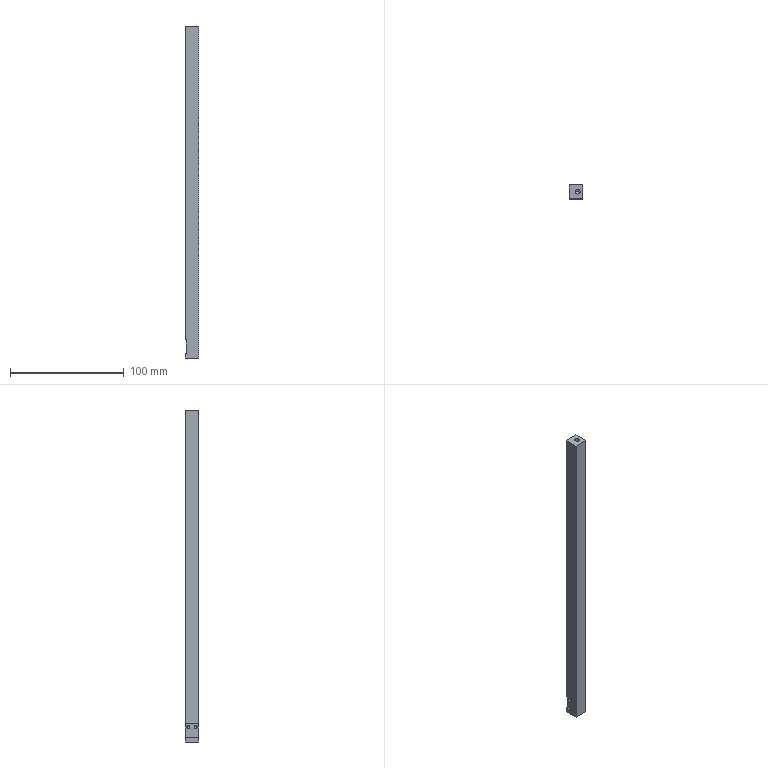Part | NX | features BREP 1 | 1 solid | 26 faces | box 12 x 12 x 292 mm | volume 41474 mm3 | plane 10 | cone 8 | cylinder 8 | commonest cylinder face diameters 2.5 x4 4.2 x4
STEP:
#1=CARTESIAN_POINT('',(-771.889,-6.832,13.662));
#2=VERTEX_POINT('',#1);
#3=CARTESIAN_POINT('',(-773.989,-6.832,12.4));
#4=VERTEX_POINT('',#3);
#5=CARTESIAN_POINT('',(-773.989,-6.832,12.4));
#6=DIRECTION('',(-0.8572,0.,-0.515));
#7=VECTOR('',#6,1000.);
#8=LINE('',#5,#7);
#9=EDGE_CURVE('',#2,#4,#8,.T.);
#10=ORIENTED_EDGE('',*,*,#9,.F.);
#11=CARTESIAN_POINT('',(-769.789,-6.832,12.4));
#12=VERTEX_POINT('',#11);
#13=CARTESIAN_POINT('',(-769.789,-6.832,12.4));
#14=DIRECTION('',(0.8572,0.,-0.515));
#15=VECTOR('',#14,1000.);
#16=LINE('',#13,#15);
#17=EDGE_CURVE('',#2,#12,#16,.T.);
#18=ORIENTED_EDGE('',*,*,#17,.T.);
#19=CARTESIAN_POINT('',(-770.231,-8.121,12.4));
#20=VERTEX_POINT('',#19);
#21=CARTESIAN_POINT('',(-771.889,-6.832,12.4));
#22=DIRECTION('',(0.,0.,-1.));
#23=DIRECTION('',(-1.,0.,0.));
#24=AXIS2_PLACEMENT_3D('',#21,#22,#23);
#25=CIRCLE('',#24,2.1);
#26=EDGE_CURVE('',#12,#20,#25,.T.);
#27=ORIENTED_EDGE('',*,*,#26,.T.);
#28=CARTESIAN_POINT('',(-773.546,-8.121,12.4));
#29=VERTEX_POINT('',#28);
#30=CARTESIAN_POINT('',(-773.546,-8.121,12.4));
#31=CARTESIAN_POINT('',(-773.126,-7.881,12.688));
#32=CARTESIAN_POINT('',(-771.895,-7.799,13.423));
#33=CARTESIAN_POINT('',(-770.654,-7.88,12.689));
#34=CARTESIAN_POINT('',(-770.231,-8.121,12.4));
#35=B_SPLINE_CURVE_WITH_KNOTS('',3,(#30,#31,#32,#33,#34),.UNSPECIFIED.,.F.,.F.,(4,1,4),(0.,0.5,1.),.UNSPECIFIED.);
#36=EDGE_CURVE('',#29,#20,#35,.T.);
#37=ORIENTED_EDGE('',*,*,#36,.F.);
#38=CARTESIAN_POINT('',(-771.889,-6.832,12.4));
#39=DIRECTION('',(0.,0.,-1.));
#40=DIRECTION('',(-1.,0.,0.));
#41=AXIS2_PLACEMENT_3D('',#38,#39,#40);
#42=CIRCLE('',#41,2.1);
#43=EDGE_CURVE('',#29,#4,#42,.T.);
#44=ORIENTED_EDGE('',*,*,#43,.T.);
#45=EDGE_LOOP('',(#10,#18,#27,#37,#44));
#46=FACE_BOUND('',#45,.T.);
#47=CARTESIAN_POINT('',(-771.889,-6.832,12.4));
#48=DIRECTION('',(0.,0.,-1.));
#49=DIRECTION('',(-1.,0.,0.));
#50=AXIS2_PLACEMENT_3D('',#47,#48,#49);
#51=CONICAL_SURFACE('',#50,2.1,1.03);
#52=ADVANCED_FACE('',(#46),#51,.F.);
#53=ORIENTED_EDGE('',*,*,#26,.F.);
#54=CARTESIAN_POINT('',(-769.789,-6.832,0.));
#55=VERTEX_POINT('',#54);
#56=CARTESIAN_POINT('',(-769.789,-6.832,0.));
#57=DIRECTION('',(0.,0.,-1.));
#58=VECTOR('',#57,1000.);
#59=LINE('',#56,#58);
#60=EDGE_CURVE('',#12,#55,#59,.T.);
#61=ORIENTED_EDGE('',*,*,#60,.T.);
#62=CARTESIAN_POINT('',(-773.989,-6.832,0.));
#63=VERTEX_POINT('',#62);
#64=CARTESIAN_POINT('',(-771.889,-6.832,0.));
#65=DIRECTION('',(0.,0.,-1.));
#66=DIRECTION('',(-1.,0.,0.));
#67=AXIS2_PLACEMENT_3D('',#64,#65,#66);
#68=CIRCLE('',#67,2.1);
#69=EDGE_CURVE('',#55,#63,#68,.T.);
#70=ORIENTED_EDGE('',*,*,#69,.T.);
#71=CARTESIAN_POINT('',(-773.989,-6.832,0.));
#72=DIRECTION('',(0.,0.,-1.));
#73=VECTOR('',#72,1000.);
#74=LINE('',#71,#73);
#75=EDGE_CURVE('',#4,#63,#74,.T.);
#76=ORIENTED_EDGE('',*,*,#75,.F.);
#77=ORIENTED_EDGE('',*,*,#43,.F.);
#78=CARTESIAN_POINT('',(-773.546,-8.121,12.4));
#79=CARTESIAN_POINT('',(-773.403,-8.305,12.179));
#80=CARTESIAN_POINT('',(-772.89,-8.778,11.952));
#81=CARTESIAN_POINT('',(-771.888,-9.009,11.963));
#82=CARTESIAN_POINT('',(-770.887,-8.777,11.952));
#83=CARTESIAN_POINT('',(-770.374,-8.305,12.179));
#84=CARTESIAN_POINT('',(-770.231,-8.121,12.4));
#85=B_SPLINE_CURVE_WITH_KNOTS('',3,(#78,#79,#80,#81,#82,#83,#84),.UNSPECIFIED.,.F.,.F.,(4,1,1,1,4),(0.,0.25,0.5,0.75,1.),.UNSPECIFIED.);
#86=EDGE_CURVE('',#20,#29,#85,.F.);
#87=ORIENTED_EDGE('',*,*,#86,.F.);
#88=EDGE_LOOP('',(#53,#61,#70,#76,#77,#87));
#89=FACE_BOUND('',#88,.T.);
#90=CARTESIAN_POINT('',(-771.889,-6.832,0.));
#91=DIRECTION('',(0.,0.,-1.));
#92=DIRECTION('',(-1.,0.,0.));
#93=AXIS2_PLACEMENT_3D('',#90,#91,#92);
#94=CYLINDRICAL_SURFACE('',#93,2.1);
#95=ADVANCED_FACE('',(#89),#94,.F.);
#96=CARTESIAN_POINT('',(-772.489,-5.832,279.6));
#97=VERTEX_POINT('',#96);
#98=CARTESIAN_POINT('',(-768.289,-5.832,279.6));
#99=VERTEX_POINT('',#98);
#100=CARTESIAN_POINT('',(-770.389,-5.832,279.6));
#101=DIRECTION('',(0.,0.,1.));
#102=DIRECTION('',(1.,0.,0.));
#103=AXIS2_PLACEMENT_3D('',#100,#101,#102);
#104=CIRCLE('',#103,2.1);
#105=EDGE_CURVE('',#97,#99,#104,.T.);
#106=ORIENTED_EDGE('',*,*,#105,.F.);
#107=CARTESIAN_POINT('',(-772.489,-5.832,292.));
#108=VERTEX_POINT('',#107);
#109=CARTESIAN_POINT('',(-772.489,-5.832,292.));
#110=DIRECTION('',(0.,0.,1.));
#111=VECTOR('',#110,1000.);
#112=LINE('',#109,#111);
#113=EDGE_CURVE('',#108,#97,#112,.F.);
#114=ORIENTED_EDGE('',*,*,#113,.F.);
#115=CARTESIAN_POINT('',(-768.289,-5.832,292.));
#116=VERTEX_POINT('',#115);
#117=CARTESIAN_POINT('',(-770.389,-5.832,292.));
#118=DIRECTION('',(0.,0.,1.));
#119=DIRECTION('',(1.,0.,0.));
#120=AXIS2_PLACEMENT_3D('',#117,#118,#119);
#121=CIRCLE('',#120,2.1);
#122=EDGE_CURVE('',#108,#116,#121,.T.);
#123=ORIENTED_EDGE('',*,*,#122,.T.);
#124=CARTESIAN_POINT('',(-768.289,-5.832,292.));
#125=DIRECTION('',(0.,0.,1.));
#126=VECTOR('',#125,1000.);
#127=LINE('',#124,#126);
#128=EDGE_CURVE('',#116,#99,#127,.F.);
#129=ORIENTED_EDGE('',*,*,#128,.T.);
#130=EDGE_LOOP('',(#106,#114,#123,#129));
#131=FACE_BOUND('',#130,.T.);
#132=CARTESIAN_POINT('',(-770.389,-5.832,292.));
#133=DIRECTION('',(0.,0.,1.));
#134=DIRECTION('',(1.,0.,0.));
#135=AXIS2_PLACEMENT_3D('',#132,#133,#134);
#136=CYLINDRICAL_SURFACE('',#135,2.1);
#137=ADVANCED_FACE('',(#131),#136,.F.);
#138=CARTESIAN_POINT('',(-770.389,-5.832,278.338));
#139=VERTEX_POINT('',#138);
#140=CARTESIAN_POINT('',(-768.289,-5.832,279.6));
#141=DIRECTION('',(0.8572,0.,0.515));
#142=VECTOR('',#141,1000.);
#143=LINE('',#140,#142);
#144=EDGE_CURVE('',#99,#139,#143,.F.);
#145=ORIENTED_EDGE('',*,*,#144,.T.);
#146=CARTESIAN_POINT('',(-772.489,-5.832,279.6));
#147=DIRECTION('',(-0.8572,0.,0.515));
#148=VECTOR('',#147,1000.);
#149=LINE('',#146,#148);
#150=EDGE_CURVE('',#97,#139,#149,.F.);
#151=ORIENTED_EDGE('',*,*,#150,.F.);
#152=ORIENTED_EDGE('',*,*,#105,.T.);
#153=EDGE_LOOP('',(#145,#151,#152));
#154=FACE_BOUND('',#153,.T.);
#155=CARTESIAN_POINT('',(-770.389,-5.832,279.6));
#156=DIRECTION('',(0.,0.,1.));
#157=DIRECTION('',(1.,0.,0.));
#158=AXIS2_PLACEMENT_3D('',#155,#156,#157);
#159=CONICAL_SURFACE('',#158,2.1,1.03);
#160=ADVANCED_FACE('',(#154),#159,.F.);
#161=CARTESIAN_POINT('',(-769.389,-9.082,11.95));
#162=VERTEX_POINT('',#161);
#163=CARTESIAN_POINT('',(-769.389,-9.082,14.45));
#164=VERTEX_POINT('',#163);
#165=CARTESIAN_POINT('',(-769.389,-9.082,13.2));
#166=DIRECTION('',(-1.,0.,0.));
#167=DIRECTION('',(0.,0.,1.));
#168=AXIS2_PLACEMENT_3D('',#165,#166,#167);
#169=CIRCLE('',#168,1.25);
#170=EDGE_CURVE('',#162,#164,#169,.T.);
#171=ORIENTED_EDGE('',*,*,#170,.F.);
#172=CARTESIAN_POINT('',(-776.889,-9.082,11.95));
#173=VERTEX_POINT('',#172);
#174=CARTESIAN_POINT('',(-776.889,-9.082,11.95));
#175=DIRECTION('',(-1.,0.,0.));
#176=VECTOR('',#175,1000.);
#177=LINE('',#174,#176);
#178=EDGE_CURVE('',#173,#162,#177,.F.);
#179=ORIENTED_EDGE('',*,*,#178,.F.);
#180=CARTESIAN_POINT('',(-776.889,-9.082,14.45));
#181=VERTEX_POINT('',#180);
#182=CARTESIAN_POINT('',(-776.889,-9.082,13.2));
#183=DIRECTION('',(-1.,0.,0.));
#184=DIRECTION('',(0.,0.,1.));
#185=AXIS2_PLACEMENT_3D('',#182,#183,#184);
#186=CIRCLE('',#185,1.25);
#187=EDGE_CURVE('',#173,#181,#186,.T.);
#188=ORIENTED_EDGE('',*,*,#187,.T.);
#189=CARTESIAN_POINT('',(-776.889,-9.082,14.45));
#190=DIRECTION('',(-1.,0.,0.));
#191=VECTOR('',#190,1000.);
#192=LINE('',#189,#191);
#193=EDGE_CURVE('',#181,#164,#192,.F.);
#194=ORIENTED_EDGE('',*,*,#193,.T.);
#195=EDGE_LOOP('',(#171,#179,#188,#194));
#196=FACE_BOUND('',#195,.T.);
#197=CARTESIAN_POINT('',(-776.889,-9.082,13.2));
#198=DIRECTION('',(-1.,0.,0.));
#199=DIRECTION('',(0.,0.,1.));
#200=AXIS2_PLACEMENT_3D('',#197,#198,#199);
#201=CYLINDRICAL_SURFACE('',#200,1.25);
#202=ADVANCED_FACE('',(#196),#201,.F.);
#203=CARTESIAN_POINT('',(-768.638,-9.082,13.2));
#204=VERTEX_POINT('',#203);
#205=CARTESIAN_POINT('',(-769.389,-9.082,14.45));
#206=DIRECTION('',(-0.515,0.,0.8572));
#207=VECTOR('',#206,1000.);
#208=LINE('',#205,#207);
#209=EDGE_CURVE('',#164,#204,#208,.F.);
#210=ORIENTED_EDGE('',*,*,#209,.T.);
#211=CARTESIAN_POINT('',(-769.389,-9.082,11.95));
#212=DIRECTION('',(-0.515,0.,-0.8572));
#213=VECTOR('',#212,1000.);
#214=LINE('',#211,#213);
#215=EDGE_CURVE('',#162,#204,#214,.F.);
#216=ORIENTED_EDGE('',*,*,#215,.F.);
#217=ORIENTED_EDGE('',*,*,#170,.T.);
#218=EDGE_LOOP('',(#210,#216,#217));
#219=FACE_BOUND('',#218,.T.);
#220=CARTESIAN_POINT('',(-769.389,-9.082,13.2));
#221=DIRECTION('',(-1.,0.,0.));
#222=DIRECTION('',(0.,0.,1.));
#223=AXIS2_PLACEMENT_3D('',#220,#221,#222);
#224=CONICAL_SURFACE('',#223,1.25,1.03);
#225=ADVANCED_FACE('',(#219),#224,.F.);
#226=CARTESIAN_POINT('',(-769.389,-2.582,11.95));
#227=VERTEX_POINT('',#226);
#228=CARTESIAN_POINT('',(-769.389,-2.582,14.45));
#229=VERTEX_POINT('',#228);
#230=CARTESIAN_POINT('',(-769.389,-2.582,13.2));
#231=DIRECTION('',(-1.,0.,0.));
#232=DIRECTION('',(0.,0.,1.));
#233=AXIS2_PLACEMENT_3D('',#230,#231,#232);
#234=CIRCLE('',#233,1.25);
#235=EDGE_CURVE('',#227,#229,#234,.T.);
#236=ORIENTED_EDGE('',*,*,#235,.F.);
#237=CARTESIAN_POINT('',(-776.889,-2.582,11.95));
#238=VERTEX_POINT('',#237);
#239=CARTESIAN_POINT('',(-776.889,-2.582,11.95));
#240=DIRECTION('',(-1.,0.,0.));
#241=VECTOR('',#240,1000.);
#242=LINE('',#239,#241);
#243=EDGE_CURVE('',#238,#227,#242,.F.);
#244=ORIENTED_EDGE('',*,*,#243,.F.);
#245=CARTESIAN_POINT('',(-776.889,-2.582,14.45));
#246=VERTEX_POINT('',#245);
#247=CARTESIAN_POINT('',(-776.889,-2.582,13.2));
#248=DIRECTION('',(-1.,0.,0.));
#249=DIRECTION('',(0.,0.,1.));
#250=AXIS2_PLACEMENT_3D('',#247,#248,#249);
#251=CIRCLE('',#250,1.25);
#252=EDGE_CURVE('',#238,#246,#251,.T.);
#253=ORIENTED_EDGE('',*,*,#252,.T.);
#254=CARTESIAN_POINT('',(-776.889,-2.582,14.45));
#255=DIRECTION('',(-1.,0.,0.));
#256=VECTOR('',#255,1000.);
#257=LINE('',#254,#256);
#258=EDGE_CURVE('',#246,#229,#257,.F.);
#259=ORIENTED_EDGE('',*,*,#258,.T.);
#260=EDGE_LOOP('',(#236,#244,#253,#259));
#261=FACE_BOUND('',#260,.T.);
#262=CARTESIAN_POINT('',(-776.889,-2.582,13.2));
#263=DIRECTION('',(-1.,0.,0.));
#264=DIRECTION('',(0.,0.,1.));
#265=AXIS2_PLACEMENT_3D('',#262,#263,#264);
#266=CYLINDRICAL_SURFACE('',#265,1.25);
#267=ADVANCED_FACE('',(#261),#266,.F.);
#268=CARTESIAN_POINT('',(-768.638,-2.582,13.2));
#269=VERTEX_POINT('',#268);
#270=CARTESIAN_POINT('',(-769.389,-2.582,14.45));
#271=DIRECTION('',(-0.515,0.,0.8572));
#272=VECTOR('',#271,1000.);
#273=LINE('',#270,#272);
#274=EDGE_CURVE('',#229,#269,#273,.F.);
#275=ORIENTED_EDGE('',*,*,#274,.T.);
#276=CARTESIAN_POINT('',(-769.389,-2.582,11.95));
#277=DIRECTION('',(-0.515,0.,-0.8572));
#278=VECTOR('',#277,1000.);
#279=LINE('',#276,#278);
#280=EDGE_CURVE('',#227,#269,#279,.F.);
#281=ORIENTED_EDGE('',*,*,#280,.F.);
#282=ORIENTED_EDGE('',*,*,#235,.T.);
#283=EDGE_LOOP('',(#275,#281,#282));
#284=FACE_BOUND('',#283,.T.);
#285=CARTESIAN_POINT('',(-769.389,-2.582,13.2));
#286=DIRECTION('',(-1.,0.,0.));
#287=DIRECTION('',(0.,0.,1.));
#288=AXIS2_PLACEMENT_3D('',#285,#286,#287);
#289=CONICAL_SURFACE('',#288,1.25,1.03);
#290=ADVANCED_FACE('',(#284),#289,.F.);
#291=CARTESIAN_POINT('',(-777.889,0.1684,292.));
#292=VERTEX_POINT('',#291);
#293=CARTESIAN_POINT('',(-777.889,0.1684,16.));
#294=VERTEX_POINT('',#293);
#295=CARTESIAN_POINT('',(-777.889,0.1684,292.));
#296=DIRECTION('',(0.,0.,-1.));
#297=VECTOR('',#296,1000.);
#298=LINE('',#295,#297);
#299=EDGE_CURVE('',#292,#294,#298,.T.);
#300=ORIENTED_EDGE('',*,*,#299,.T.);
#301=CARTESIAN_POINT('',(-777.889,-11.832,16.));
#302=VERTEX_POINT('',#301);
#303=CARTESIAN_POINT('',(-777.889,0.1684,16.));
#304=DIRECTION('',(0.,-1.,0.));
#305=VECTOR('',#304,1000.);
#306=LINE('',#303,#305);
#307=EDGE_CURVE('',#294,#302,#306,.T.);
#308=ORIENTED_EDGE('',*,*,#307,.T.);
#309=CARTESIAN_POINT('',(-777.889,-11.832,292.));
#310=VERTEX_POINT('',#309);
#311=CARTESIAN_POINT('',(-777.889,-11.832,292.));
#312=DIRECTION('',(0.,0.,-1.));
#313=VECTOR('',#312,1000.);
#314=LINE('',#311,#313);
#315=EDGE_CURVE('',#310,#302,#314,.T.);
#316=ORIENTED_EDGE('',*,*,#315,.F.);
#317=CARTESIAN_POINT('',(-777.889,-11.832,292.));
#318=DIRECTION('',(0.,-1.,0.));
#319=VECTOR('',#318,1000.);
#320=LINE('',#317,#319);
#321=EDGE_CURVE('',#292,#310,#320,.T.);
#322=ORIENTED_EDGE('',*,*,#321,.F.);
#323=EDGE_LOOP('',(#300,#308,#316,#322));
#324=FACE_BOUND('',#323,.T.);
#325=CARTESIAN_POINT('',(-777.889,-11.832,292.));
#326=DIRECTION('',(1.,0.,0.));
#327=DIRECTION('',(0.,1.,0.));
#328=AXIS2_PLACEMENT_3D('',#325,#326,#327);
#329=PLANE('',#328);
#330=ADVANCED_FACE('',(#324),#329,.F.);
#331=CARTESIAN_POINT('',(-765.889,-11.832,0.));
#332=VERTEX_POINT('',#331);
#333=CARTESIAN_POINT('',(-765.889,0.1684,0.));
#334=VERTEX_POINT('',#333);
#335=CARTESIAN_POINT('',(-765.889,-11.832,0.));
#336=DIRECTION('',(0.,1.,0.));
#337=VECTOR('',#336,1000.);
#338=LINE('',#335,#337);
#339=EDGE_CURVE('',#332,#334,#338,.T.);
#340=ORIENTED_EDGE('',*,*,#339,.T.);
#341=CARTESIAN_POINT('',(-765.889,0.1684,292.));
#342=VERTEX_POINT('',#341);
#343=CARTESIAN_POINT('',(-765.889,0.1684,292.));
#344=DIRECTION('',(0.,0.,-1.));
#345=VECTOR('',#344,1000.);
#346=LINE('',#343,#345);
#347=EDGE_CURVE('',#342,#334,#346,.T.);
#348=ORIENTED_EDGE('',*,*,#347,.F.);
#349=CARTESIAN_POINT('',(-765.889,-11.832,292.));
#350=VERTEX_POINT('',#349);
#351=CARTESIAN_POINT('',(-765.889,-11.832,292.));
#352=DIRECTION('',(0.,1.,0.));
#353=VECTOR('',#352,1000.);
#354=LINE('',#351,#353);
#355=EDGE_CURVE('',#350,#342,#354,.T.);
#356=ORIENTED_EDGE('',*,*,#355,.F.);
#357=CARTESIAN_POINT('',(-765.889,-11.832,292.));
#358=DIRECTION('',(0.,0.,-1.));
#359=VECTOR('',#358,1000.);
#360=LINE('',#357,#359);
#361=EDGE_CURVE('',#350,#332,#360,.T.);
#362=ORIENTED_EDGE('',*,*,#361,.T.);
#363=EDGE_LOOP('',(#340,#348,#356,#362));
#364=FACE_BOUND('',#363,.T.);
#365=CARTESIAN_POINT('',(-765.889,-11.832,292.));
#366=DIRECTION('',(-1.,0.,0.));
#367=DIRECTION('',(0.,0.,1.));
#368=AXIS2_PLACEMENT_3D('',#365,#366,#367);
#369=PLANE('',#368);
#370=ADVANCED_FACE('',(#364),#369,.F.);
#371=CARTESIAN_POINT('',(-776.889,0.1684,4.));
#372=VERTEX_POINT('',#371);
#373=CARTESIAN_POINT('',(-776.889,0.1684,16.));
#374=VERTEX_POINT('',#373);
#375=CARTESIAN_POINT('',(-776.889,0.1684,16.));
#376=DIRECTION('',(0.,0.,1.));
#377=VECTOR('',#376,1000.);
#378=LINE('',#375,#377);
#379=EDGE_CURVE('',#372,#374,#378,.T.);
#380=ORIENTED_EDGE('',*,*,#379,.T.);
#381=CARTESIAN_POINT('',(-777.889,0.1684,16.));
#382=DIRECTION('',(-1.,0.,0.));
#383=VECTOR('',#382,1000.);
#384=LINE('',#381,#383);
#385=EDGE_CURVE('',#374,#294,#384,.T.);
#386=ORIENTED_EDGE('',*,*,#385,.T.);
#387=ORIENTED_EDGE('',*,*,#299,.F.);
#388=CARTESIAN_POINT('',(-765.889,0.1684,292.));
#389=DIRECTION('',(-1.,0.,0.));
#390=VECTOR('',#389,1000.);
#391=LINE('',#388,#390);
#392=EDGE_CURVE('',#342,#292,#391,.T.);
#393=ORIENTED_EDGE('',*,*,#392,.F.);
#394=ORIENTED_EDGE('',*,*,#347,.T.);
#395=CARTESIAN_POINT('',(-777.889,0.1684,0.));
#396=VERTEX_POINT('',#395);
#397=CARTESIAN_POINT('',(-765.889,0.1684,0.));
#398=DIRECTION('',(-1.,0.,0.));
#399=VECTOR('',#398,1000.);
#400=LINE('',#397,#399);
#401=EDGE_CURVE('',#334,#396,#400,.T.);
#402=ORIENTED_EDGE('',*,*,#401,.T.);
#403=CARTESIAN_POINT('',(-777.889,0.1684,4.));
#404=VERTEX_POINT('',#403);
#405=CARTESIAN_POINT('',(-777.889,0.1684,292.));
#406=DIRECTION('',(0.,0.,-1.));
#407=VECTOR('',#406,1000.);
#408=LINE('',#405,#407);
#409=EDGE_CURVE('',#404,#396,#408,.T.);
#410=ORIENTED_EDGE('',*,*,#409,.F.);
#411=CARTESIAN_POINT('',(-777.889,0.1684,4.));
#412=DIRECTION('',(1.,0.,0.));
#413=VECTOR('',#412,1000.);
#414=LINE('',#411,#413);
#415=EDGE_CURVE('',#404,#372,#414,.T.);
#416=ORIENTED_EDGE('',*,*,#415,.T.);
#417=EDGE_LOOP('',(#380,#386,#387,#393,#394,#402,#410,#416));
#418=FACE_BOUND('',#417,.T.);
#419=CARTESIAN_POINT('',(-765.889,0.1684,292.));
#420=DIRECTION('',(0.,-1.,0.));
#421=DIRECTION('',(0.,0.,-1.));
#422=AXIS2_PLACEMENT_3D('',#419,#420,#421);
#423=PLANE('',#422);
#424=ADVANCED_FACE('',(#418),#423,.F.);
#425=CARTESIAN_POINT('',(-777.889,-11.832,4.));
#426=VERTEX_POINT('',#425);
#427=CARTESIAN_POINT('',(-777.889,-11.832,0.));
#428=VERTEX_POINT('',#427);
#429=CARTESIAN_POINT('',(-777.889,-11.832,292.));
#430=DIRECTION('',(0.,0.,-1.));
#431=VECTOR('',#430,1000.);
#432=LINE('',#429,#431);
#433=EDGE_CURVE('',#426,#428,#432,.T.);
#434=ORIENTED_EDGE('',*,*,#433,.F.);
#435=CARTESIAN_POINT('',(-777.889,0.1684,4.));
#436=DIRECTION('',(0.,-1.,0.));
#437=VECTOR('',#436,1000.);
#438=LINE('',#435,#437);
#439=EDGE_CURVE('',#404,#426,#438,.T.);
#440=ORIENTED_EDGE('',*,*,#439,.F.);
#441=ORIENTED_EDGE('',*,*,#409,.T.);
#442=CARTESIAN_POINT('',(-777.889,-11.832,0.));
#443=DIRECTION('',(0.,-1.,0.));
#444=VECTOR('',#443,1000.);
#445=LINE('',#442,#444);
#446=EDGE_CURVE('',#396,#428,#445,.T.);
#447=ORIENTED_EDGE('',*,*,#446,.T.);
#448=EDGE_LOOP('',(#434,#440,#441,#447));
#449=FACE_BOUND('',#448,.T.);
#450=CARTESIAN_POINT('',(-777.889,-11.832,292.));
#451=DIRECTION('',(1.,0.,0.));
#452=DIRECTION('',(0.,1.,0.));
#453=AXIS2_PLACEMENT_3D('',#450,#451,#452);
#454=PLANE('',#453);
#455=ADVANCED_FACE('',(#449),#454,.F.);
#456=ORIENTED_EDGE('',*,*,#315,.T.);
#457=CARTESIAN_POINT('',(-776.889,-11.832,16.));
#458=VERTEX_POINT('',#457);
#459=CARTESIAN_POINT('',(-777.889,-11.832,16.));
#460=DIRECTION('',(-1.,0.,0.));
#461=VECTOR('',#460,1000.);
#462=LINE('',#459,#461);
#463=EDGE_CURVE('',#458,#302,#462,.T.);
#464=ORIENTED_EDGE('',*,*,#463,.F.);
#465=CARTESIAN_POINT('',(-776.889,-11.832,4.));
#466=VERTEX_POINT('',#465);
#467=CARTESIAN_POINT('',(-776.889,-11.832,16.));
#468=DIRECTION('',(0.,0.,1.));
#469=VECTOR('',#468,1000.);
#470=LINE('',#467,#469);
#471=EDGE_CURVE('',#466,#458,#470,.T.);
#472=ORIENTED_EDGE('',*,*,#471,.F.);
#473=CARTESIAN_POINT('',(-777.889,-11.832,4.));
#474=DIRECTION('',(1.,0.,0.));
#475=VECTOR('',#474,1000.);
#476=LINE('',#473,#475);
#477=EDGE_CURVE('',#426,#466,#476,.T.);
#478=ORIENTED_EDGE('',*,*,#477,.F.);
#479=ORIENTED_EDGE('',*,*,#433,.T.);
#480=CARTESIAN_POINT('',(-765.889,-11.832,0.));
#481=DIRECTION('',(1.,0.,0.));
#482=VECTOR('',#481,1000.);
#483=LINE('',#480,#482);
#484=EDGE_CURVE('',#428,#332,#483,.T.);
#485=ORIENTED_EDGE('',*,*,#484,.T.);
#486=ORIENTED_EDGE('',*,*,#361,.F.);
#487=CARTESIAN_POINT('',(-765.889,-11.832,292.));
#488=DIRECTION('',(1.,0.,0.));
#489=VECTOR('',#488,1000.);
#490=LINE('',#487,#489);
#491=EDGE_CURVE('',#310,#350,#490,.T.);
#492=ORIENTED_EDGE('',*,*,#491,.F.);
#493=EDGE_LOOP('',(#456,#464,#472,#478,#479,#485,#486,#492));
#494=FACE_BOUND('',#493,.T.);
#495=CARTESIAN_POINT('',(-765.889,-11.832,292.));
#496=DIRECTION('',(0.,1.,0.));
#497=DIRECTION('',(1.,0.,0.));
#498=AXIS2_PLACEMENT_3D('',#495,#496,#497);
#499=PLANE('',#498);
#500=ADVANCED_FACE('',(#494),#499,.F.);
#501=ORIENTED_EDGE('',*,*,#355,.T.);
#502=ORIENTED_EDGE('',*,*,#392,.T.);
#503=ORIENTED_EDGE('',*,*,#321,.T.);
#504=ORIENTED_EDGE('',*,*,#491,.T.);
#505=EDGE_LOOP('',(#501,#502,#503,#504));
#506=FACE_BOUND('',#505,.T.);
#507=CARTESIAN_POINT('',(-770.389,-5.832,292.));
#508=DIRECTION('',(0.,0.,1.));
#509=DIRECTION('',(1.,0.,0.));
#510=AXIS2_PLACEMENT_3D('',#507,#508,#509);
#511=CIRCLE('',#510,2.1);
#512=EDGE_CURVE('',#116,#108,#511,.T.);
#513=ORIENTED_EDGE('',*,*,#512,.F.);
#514=ORIENTED_EDGE('',*,*,#122,.F.);
#515=EDGE_LOOP('',(#513,#514));
#516=FACE_BOUND('',#515,.T.);
#517=CARTESIAN_POINT('',(-765.889,0.1684,292.));
#518=DIRECTION('',(0.,0.,1.));
#519=DIRECTION('',(1.,0.,0.));
#520=AXIS2_PLACEMENT_3D('',#517,#518,#519);
#521=PLANE('',#520);
#522=ADVANCED_FACE('',(#506,#516),#521,.T.);
#523=ORIENTED_EDGE('',*,*,#339,.F.);
#524=ORIENTED_EDGE('',*,*,#484,.F.);
#525=ORIENTED_EDGE('',*,*,#446,.F.);
#526=ORIENTED_EDGE('',*,*,#401,.F.);
#527=EDGE_LOOP('',(#523,#524,#525,#526));
#528=FACE_BOUND('',#527,.T.);
#529=CARTESIAN_POINT('',(-771.889,-6.832,0.));
#530=DIRECTION('',(0.,0.,-1.));
#531=DIRECTION('',(-1.,0.,0.));
#532=AXIS2_PLACEMENT_3D('',#529,#530,#531);
#533=CIRCLE('',#532,2.1);
#534=EDGE_CURVE('',#63,#55,#533,.T.);
#535=ORIENTED_EDGE('',*,*,#534,.F.);
#536=ORIENTED_EDGE('',*,*,#69,.F.);
#537=EDGE_LOOP('',(#535,#536));
#538=FACE_BOUND('',#537,.T.);
#539=CARTESIAN_POINT('',(-765.889,0.1684,0.));
#540=DIRECTION('',(0.,0.,1.));
#541=DIRECTION('',(1.,0.,0.));
#542=AXIS2_PLACEMENT_3D('',#539,#540,#541);
#543=PLANE('',#542);
#544=ADVANCED_FACE('',(#528,#538),#543,.F.);
#545=ORIENTED_EDGE('',*,*,#463,.T.);
#546=ORIENTED_EDGE('',*,*,#307,.F.);
#547=ORIENTED_EDGE('',*,*,#385,.F.);
#548=CARTESIAN_POINT('',(-776.889,0.1684,16.));
#549=DIRECTION('',(0.,-1.,0.));
#550=VECTOR('',#549,1000.);
#551=LINE('',#548,#550);
#552=EDGE_CURVE('',#374,#458,#551,.T.);
#553=ORIENTED_EDGE('',*,*,#552,.T.);
#554=EDGE_LOOP('',(#545,#546,#547,#553));
#555=FACE_BOUND('',#554,.T.);
#556=CARTESIAN_POINT('',(-777.889,0.1684,16.));
#557=DIRECTION('',(0.,0.,1.));
#558=DIRECTION('',(1.,0.,0.));
#559=AXIS2_PLACEMENT_3D('',#556,#557,#558);
#560=PLANE('',#559);
#561=ADVANCED_FACE('',(#555),#560,.F.);
#562=ORIENTED_EDGE('',*,*,#471,.T.);
#563=ORIENTED_EDGE('',*,*,#552,.F.);
#564=ORIENTED_EDGE('',*,*,#379,.F.);
#565=CARTESIAN_POINT('',(-776.889,0.1684,4.));
#566=DIRECTION('',(0.,-1.,0.));
#567=VECTOR('',#566,1000.);
#568=LINE('',#565,#567);
#569=EDGE_CURVE('',#372,#466,#568,.T.);
#570=ORIENTED_EDGE('',*,*,#569,.T.);
#571=EDGE_LOOP('',(#562,#563,#564,#570));
#572=FACE_BOUND('',#571,.T.);
#573=CARTESIAN_POINT('',(-776.889,-9.082,13.2));
#574=DIRECTION('',(-1.,0.,0.));
#575=DIRECTION('',(0.,0.,1.));
#576=AXIS2_PLACEMENT_3D('',#573,#574,#575);
#577=CIRCLE('',#576,1.25);
#578=EDGE_CURVE('',#181,#173,#577,.T.);
#579=ORIENTED_EDGE('',*,*,#578,.F.);
#580=ORIENTED_EDGE('',*,*,#187,.F.);
#581=EDGE_LOOP('',(#579,#580));
#582=FACE_BOUND('',#581,.T.);
#583=CARTESIAN_POINT('',(-776.889,-2.582,13.2));
#584=DIRECTION('',(-1.,0.,0.));
#585=DIRECTION('',(0.,0.,1.));
#586=AXIS2_PLACEMENT_3D('',#583,#584,#585);
#587=CIRCLE('',#586,1.25);
#588=EDGE_CURVE('',#246,#238,#587,.T.);
#589=ORIENTED_EDGE('',*,*,#588,.F.);
#590=ORIENTED_EDGE('',*,*,#252,.F.);
#591=EDGE_LOOP('',(#589,#590));
#592=FACE_BOUND('',#591,.T.);
#593=CARTESIAN_POINT('',(-776.889,0.1684,16.));
#594=DIRECTION('',(1.,0.,0.));
#595=DIRECTION('',(0.,1.,0.));
#596=AXIS2_PLACEMENT_3D('',#593,#594,#595);
#597=PLANE('',#596);
#598=ADVANCED_FACE('',(#572,#582,#592),#597,.F.);
#599=ORIENTED_EDGE('',*,*,#477,.T.);
#600=ORIENTED_EDGE('',*,*,#569,.F.);
#601=ORIENTED_EDGE('',*,*,#415,.F.);
#602=ORIENTED_EDGE('',*,*,#439,.T.);
#603=EDGE_LOOP('',(#599,#600,#601,#602));
#604=FACE_BOUND('',#603,.T.);
#605=CARTESIAN_POINT('',(-777.889,0.1684,4.));
#606=DIRECTION('',(0.,0.,-1.));
#607=DIRECTION('',(0.,-1.,0.));
#608=AXIS2_PLACEMENT_3D('',#605,#606,#607);
#609=PLANE('',#608);
#610=ADVANCED_FACE('',(#604),#609,.F.);
#611=ORIENTED_EDGE('',*,*,#280,.T.);
#612=ORIENTED_EDGE('',*,*,#274,.F.);
#613=CARTESIAN_POINT('',(-769.389,-2.582,13.2));
#614=DIRECTION('',(-1.,0.,0.));
#615=DIRECTION('',(0.,0.,1.));
#616=AXIS2_PLACEMENT_3D('',#613,#614,#615);
#617=CIRCLE('',#616,1.25);
#618=EDGE_CURVE('',#229,#227,#617,.T.);
#619=ORIENTED_EDGE('',*,*,#618,.T.);
#620=EDGE_LOOP('',(#611,#612,#619));
#621=FACE_BOUND('',#620,.T.);
#622=CARTESIAN_POINT('',(-769.389,-2.582,13.2));
#623=DIRECTION('',(-1.,0.,0.));
#624=DIRECTION('',(0.,0.,1.));
#625=AXIS2_PLACEMENT_3D('',#622,#623,#624);
#626=CONICAL_SURFACE('',#625,1.25,1.03);
#627=ADVANCED_FACE('',(#621),#626,.F.);
#628=ORIENTED_EDGE('',*,*,#243,.T.);
#629=ORIENTED_EDGE('',*,*,#618,.F.);
#630=ORIENTED_EDGE('',*,*,#258,.F.);
#631=ORIENTED_EDGE('',*,*,#588,.T.);
#632=EDGE_LOOP('',(#628,#629,#630,#631));
#633=FACE_BOUND('',#632,.T.);
#634=CARTESIAN_POINT('',(-776.889,-2.582,13.2));
#635=DIRECTION('',(-1.,0.,0.));
#636=DIRECTION('',(0.,0.,1.));
#637=AXIS2_PLACEMENT_3D('',#634,#635,#636);
#638=CYLINDRICAL_SURFACE('',#637,1.25);
#639=ADVANCED_FACE('',(#633),#638,.F.);
#640=ORIENTED_EDGE('',*,*,#215,.T.);
#641=ORIENTED_EDGE('',*,*,#209,.F.);
#642=CARTESIAN_POINT('',(-769.389,-9.082,13.2));
#643=DIRECTION('',(-1.,0.,0.));
#644=DIRECTION('',(0.,0.,1.));
#645=AXIS2_PLACEMENT_3D('',#642,#643,#644);
#646=CIRCLE('',#645,1.25);
#647=EDGE_CURVE('',#164,#162,#646,.T.);
#648=ORIENTED_EDGE('',*,*,#647,.T.);
#649=EDGE_LOOP('',(#640,#641,#648));
#650=FACE_BOUND('',#649,.T.);
#651=CARTESIAN_POINT('',(-769.389,-9.082,13.2));
#652=DIRECTION('',(-1.,0.,0.));
#653=DIRECTION('',(0.,0.,1.));
#654=AXIS2_PLACEMENT_3D('',#651,#652,#653);
#655=CONICAL_SURFACE('',#654,1.25,1.03);
#656=ADVANCED_FACE('',(#650),#655,.F.);
#657=ORIENTED_EDGE('',*,*,#178,.T.);
#658=ORIENTED_EDGE('',*,*,#647,.F.);
#659=ORIENTED_EDGE('',*,*,#193,.F.);
#660=ORIENTED_EDGE('',*,*,#578,.T.);
#661=EDGE_LOOP('',(#657,#658,#659,#660));
#662=FACE_BOUND('',#661,.T.);
#663=ORIENTED_EDGE('',*,*,#36,.T.);
#664=ORIENTED_EDGE('',*,*,#86,.T.);
#665=EDGE_LOOP('',(#663,#664));
#666=FACE_BOUND('',#665,.T.);
#667=CARTESIAN_POINT('',(-776.889,-9.082,13.2));
#668=DIRECTION('',(-1.,0.,0.));
#669=DIRECTION('',(0.,0.,1.));
#670=AXIS2_PLACEMENT_3D('',#667,#668,#669);
#671=CYLINDRICAL_SURFACE('',#670,1.25);
#672=ADVANCED_FACE('',(#662,#666),#671,.F.);
#673=ORIENTED_EDGE('',*,*,#150,.T.);
#674=ORIENTED_EDGE('',*,*,#144,.F.);
#675=CARTESIAN_POINT('',(-770.389,-5.832,279.6));
#676=DIRECTION('',(0.,0.,1.));
#677=DIRECTION('',(1.,0.,0.));
#678=AXIS2_PLACEMENT_3D('',#675,#676,#677);
#679=CIRCLE('',#678,2.1);
#680=EDGE_CURVE('',#99,#97,#679,.T.);
#681=ORIENTED_EDGE('',*,*,#680,.T.);
#682=EDGE_LOOP('',(#673,#674,#681));
#683=FACE_BOUND('',#682,.T.);
#684=CARTESIAN_POINT('',(-770.389,-5.832,279.6));
#685=DIRECTION('',(0.,0.,1.));
#686=DIRECTION('',(1.,0.,0.));
#687=AXIS2_PLACEMENT_3D('',#684,#685,#686);
#688=CONICAL_SURFACE('',#687,2.1,1.03);
#689=ADVANCED_FACE('',(#683),#688,.F.);
#690=ORIENTED_EDGE('',*,*,#113,.T.);
#691=ORIENTED_EDGE('',*,*,#680,.F.);
#692=ORIENTED_EDGE('',*,*,#128,.F.);
#693=ORIENTED_EDGE('',*,*,#512,.T.);
#694=EDGE_LOOP('',(#690,#691,#692,#693));
#695=FACE_BOUND('',#694,.T.);
#696=CARTESIAN_POINT('',(-770.389,-5.832,292.));
#697=DIRECTION('',(0.,0.,1.));
#698=DIRECTION('',(1.,0.,0.));
#699=AXIS2_PLACEMENT_3D('',#696,#697,#698);
#700=CYLINDRICAL_SURFACE('',#699,2.1);
#701=ADVANCED_FACE('',(#695),#700,.F.);
#702=ORIENTED_EDGE('',*,*,#60,.F.);
#703=CARTESIAN_POINT('',(-771.889,-6.832,12.4));
#704=DIRECTION('',(0.,0.,-1.));
#705=DIRECTION('',(-1.,0.,0.));
#706=AXIS2_PLACEMENT_3D('',#703,#704,#705);
#707=CIRCLE('',#706,2.1);
#708=EDGE_CURVE('',#4,#12,#707,.T.);
#709=ORIENTED_EDGE('',*,*,#708,.F.);
#710=ORIENTED_EDGE('',*,*,#75,.T.);
#711=ORIENTED_EDGE('',*,*,#534,.T.);
#712=EDGE_LOOP('',(#702,#709,#710,#711));
#713=FACE_BOUND('',#712,.T.);
#714=CARTESIAN_POINT('',(-771.889,-6.832,0.));
#715=DIRECTION('',(0.,0.,-1.));
#716=DIRECTION('',(-1.,0.,0.));
#717=AXIS2_PLACEMENT_3D('',#714,#715,#716);
#718=CYLINDRICAL_SURFACE('',#717,2.1);
#719=ADVANCED_FACE('',(#713),#718,.F.);
#720=ORIENTED_EDGE('',*,*,#17,.F.);
#721=ORIENTED_EDGE('',*,*,#9,.T.);
#722=ORIENTED_EDGE('',*,*,#708,.T.);
#723=EDGE_LOOP('',(#720,#721,#722));
#724=FACE_BOUND('',#723,.T.);
#725=CARTESIAN_POINT('',(-771.889,-6.832,12.4));
#726=DIRECTION('',(0.,0.,-1.));
#727=DIRECTION('',(-1.,0.,0.));
#728=AXIS2_PLACEMENT_3D('',#725,#726,#727);
#729=CONICAL_SURFACE('',#728,2.1,1.03);
#730=ADVANCED_FACE('',(#724),#729,.F.);
#731=CLOSED_SHELL('',(#52,#95,#137,#160,#202,#225,#267,#290,#330,#370,#424,#455,#500,#522,#544,#561,#598,#610,#627,#639,#656,#672,#689,#701,#719,#730));
#732=MANIFOLD_SOLID_BREP('',#731);
#733=(LENGTH_UNIT()NAMED_UNIT(*)SI_UNIT(.MILLI.,.METRE.));
#734=UNCERTAINTY_MEASURE_WITH_UNIT(LENGTH_MEASURE(0.0508),#733,'','');
#735=(NAMED_UNIT(*)PLANE_ANGLE_UNIT()SI_UNIT($,.RADIAN.));
#736=(NAMED_UNIT(*)SI_UNIT($,.STERADIAN.)SOLID_ANGLE_UNIT());
#737=(GEOMETRIC_REPRESENTATION_CONTEXT(3)GLOBAL_UNCERTAINTY_ASSIGNED_CONTEXT((#734))GLOBAL_UNIT_ASSIGNED_CONTEXT((#733,#735,#736))REPRESENTATION_CONTEXT('',''));
#738=ADVANCED_BREP_SHAPE_REPRESENTATION('',(#732),#737);